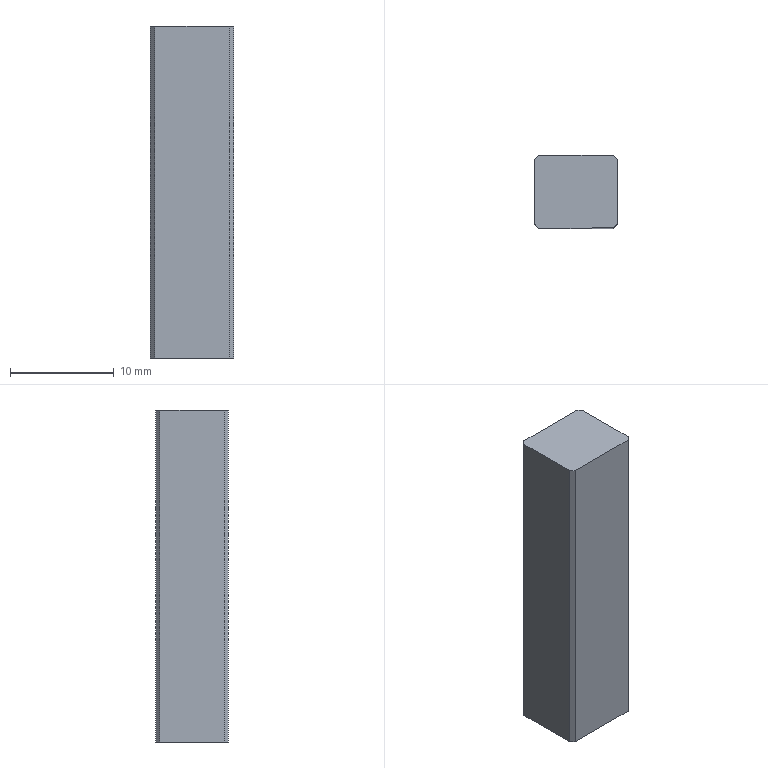Part | STEP file | PLAIN_PARALLEL_KEYS-1-SOLID1 | 1 solid | 10 faces | box 8.009 x 7.011 x 32 mm | volume 1782 mm3 | plane 10
STEP:
#1=CARTESIAN_POINT('',(0.,0.,0.));
#2=DIRECTION('',(0.,0.,1.));
#3=DIRECTION('',(1.,0.,0.));
#4=AXIS2_PLACEMENT_3D('',#1,#2,#3);
#5=CARTESIAN_POINT('',(-3.61,6.995,55.));
#6=VERTEX_POINT('',#5);
#7=CARTESIAN_POINT('',(-3.61,6.995,23.));
#8=VERTEX_POINT('',#7);
#9=CARTESIAN_POINT('',(-3.61,6.995,51.));
#10=DIRECTION('',(0.,0.,-1.));
#11=VECTOR('',#10,1.);
#12=LINE('',#9,#11);
#13=CARTESIAN_POINT('',(-0.01045,7.,51.));
#14=DIRECTION('',(0.001493,-1.,0.));
#15=DIRECTION('',(1.,0.001493,0.));
#16=AXIS2_PLACEMENT_3D('',#13,#14,#15);
#17=PLANE('',#16);
#18=CARTESIAN_POINT('',(-3.6,0.));
#19=DIRECTION('',(0.,-1.));
#20=VECTOR('',#19,1.);
#21=LINE('',#18,#20);
#22=(GEOMETRIC_REPRESENTATION_CONTEXT(2)PARAMETRIC_REPRESENTATION_CONTEXT()REPRESENTATION_CONTEXT('',''));
#23=DEFINITIONAL_REPRESENTATION('',(#21),#22);
#24=PCURVE('',#17,#23);
#25=CARTESIAN_POINT('',(-4.011,7.394,51.));
#26=DIRECTION('',(-0.7061,-0.7082,0.));
#27=DIRECTION('',(0.7082,-0.7061,0.));
#28=AXIS2_PLACEMENT_3D('',#25,#26,#27);
#29=PLANE('',#28);
#30=CARTESIAN_POINT('',(0.5657,0.));
#31=DIRECTION('',(0.,-1.));
#32=VECTOR('',#31,1.);
#33=LINE('',#30,#32);
#34=(GEOMETRIC_REPRESENTATION_CONTEXT(2)PARAMETRIC_REPRESENTATION_CONTEXT()REPRESENTATION_CONTEXT('',''));
#35=DEFINITIONAL_REPRESENTATION('',(#33),#34);
#36=PCURVE('',#29,#35);
#37=SURFACE_CURVE('',#12,(#24,#36),.PCURVE_S1.);
#38=EDGE_CURVE('',#6,#8,#37,.T.);
#39=ORIENTED_EDGE('',*,*,#38,.T.);
#40=CARTESIAN_POINT('',(3.59,7.005,23.));
#41=VERTEX_POINT('',#40);
#42=CARTESIAN_POINT('',(-0.01045,7.,23.));
#43=DIRECTION('',(1.,0.001493,0.));
#44=VECTOR('',#43,1.);
#45=LINE('',#42,#44);
#46=CARTESIAN_POINT('',(0.,-28.));
#47=DIRECTION('',(1.,0.));
#48=VECTOR('',#47,1.);
#49=LINE('',#46,#48);
#50=(GEOMETRIC_REPRESENTATION_CONTEXT(2)PARAMETRIC_REPRESENTATION_CONTEXT()REPRESENTATION_CONTEXT('',''));
#51=DEFINITIONAL_REPRESENTATION('',(#49),#50);
#52=PCURVE('',#17,#51);
#53=CARTESIAN_POINT('',(-4.021,13.994,23.));
#54=DIRECTION('',(0.,0.,1.));
#55=DIRECTION('',(1.,0.,0.));
#56=AXIS2_PLACEMENT_3D('',#53,#54,#55);
#57=PLANE('',#56);
#58=CARTESIAN_POINT('',(4.01,-6.994));
#59=DIRECTION('',(1.,0.001493));
#60=VECTOR('',#59,1.);
#61=LINE('',#58,#60);
#62=(GEOMETRIC_REPRESENTATION_CONTEXT(2)PARAMETRIC_REPRESENTATION_CONTEXT()REPRESENTATION_CONTEXT('',''));
#63=DEFINITIONAL_REPRESENTATION('',(#61),#62);
#64=PCURVE('',#57,#63);
#65=SURFACE_CURVE('',#45,(#52,#64),.PCURVE_S1.);
#66=EDGE_CURVE('',#8,#41,#65,.T.);
#67=ORIENTED_EDGE('',*,*,#66,.T.);
#68=CARTESIAN_POINT('',(3.59,7.005,55.));
#69=VERTEX_POINT('',#68);
#70=CARTESIAN_POINT('',(3.59,7.005,51.));
#71=DIRECTION('',(0.,0.,1.));
#72=VECTOR('',#71,1.);
#73=LINE('',#70,#72);
#74=CARTESIAN_POINT('',(3.6,0.));
#75=DIRECTION('',(0.,1.));
#76=VECTOR('',#75,1.);
#77=LINE('',#74,#76);
#78=(GEOMETRIC_REPRESENTATION_CONTEXT(2)PARAMETRIC_REPRESENTATION_CONTEXT()REPRESENTATION_CONTEXT('',''));
#79=DEFINITIONAL_REPRESENTATION('',(#77),#78);
#80=PCURVE('',#17,#79);
#81=CARTESIAN_POINT('',(3.989,7.406,27.));
#82=DIRECTION('',(0.7082,-0.7061,0.));
#83=DIRECTION('',(0.7061,0.7082,0.));
#84=AXIS2_PLACEMENT_3D('',#81,#82,#83);
#85=PLANE('',#84);
#86=CARTESIAN_POINT('',(-0.5657,24.));
#87=DIRECTION('',(0.,1.));
#88=VECTOR('',#87,1.);
#89=LINE('',#86,#88);
#90=(GEOMETRIC_REPRESENTATION_CONTEXT(2)PARAMETRIC_REPRESENTATION_CONTEXT()REPRESENTATION_CONTEXT('',''));
#91=DEFINITIONAL_REPRESENTATION('',(#89),#90);
#92=PCURVE('',#85,#91);
#93=SURFACE_CURVE('',#73,(#80,#92),.PCURVE_S1.);
#94=EDGE_CURVE('',#41,#69,#93,.T.);
#95=ORIENTED_EDGE('',*,*,#94,.T.);
#96=CARTESIAN_POINT('',(-0.01045,7.,55.));
#97=DIRECTION('',(-1.,-0.001493,0.));
#98=VECTOR('',#97,1.);
#99=LINE('',#96,#98);
#100=CARTESIAN_POINT('',(0.,4.));
#101=DIRECTION('',(-1.,0.));
#102=VECTOR('',#101,1.);
#103=LINE('',#100,#102);
#104=(GEOMETRIC_REPRESENTATION_CONTEXT(2)PARAMETRIC_REPRESENTATION_CONTEXT()REPRESENTATION_CONTEXT('',''));
#105=DEFINITIONAL_REPRESENTATION('',(#103),#104);
#106=PCURVE('',#17,#105);
#107=CARTESIAN_POINT('',(-4.021,13.994,55.));
#108=DIRECTION('',(0.,0.,-1.));
#109=DIRECTION('',(-1.,0.,0.));
#110=AXIS2_PLACEMENT_3D('',#107,#108,#109);
#111=PLANE('',#110);
#112=CARTESIAN_POINT('',(-4.01,-6.994));
#113=DIRECTION('',(1.,-0.001493));
#114=VECTOR('',#113,1.);
#115=LINE('',#112,#114);
#116=(GEOMETRIC_REPRESENTATION_CONTEXT(2)PARAMETRIC_REPRESENTATION_CONTEXT()REPRESENTATION_CONTEXT('',''));
#117=DEFINITIONAL_REPRESENTATION('',(#115),#116);
#118=PCURVE('',#111,#117);
#119=SURFACE_CURVE('',#99,(#106,#118),.PCURVE_S1.);
#120=EDGE_CURVE('',#69,#6,#119,.T.);
#121=ORIENTED_EDGE('',*,*,#120,.T.);
#122=EDGE_LOOP('',(#39,#67,#95,#121));
#123=FACE_BOUND('',#122,.T.);
#124=ADVANCED_FACE('',(#123),#17,.T.);
#125=ORIENTED_EDGE('',*,*,#66,.F.);
#126=CARTESIAN_POINT('',(-4.011,7.394,23.));
#127=VERTEX_POINT('',#126);
#128=CARTESIAN_POINT('',(-4.011,7.394,23.));
#129=DIRECTION('',(0.7082,-0.7061,0.));
#130=VECTOR('',#129,1.);
#131=LINE('',#128,#130);
#132=CARTESIAN_POINT('',(0.009856,-6.6));
#133=DIRECTION('',(0.7082,-0.7061));
#134=VECTOR('',#133,1.);
#135=LINE('',#132,#134);
#136=(GEOMETRIC_REPRESENTATION_CONTEXT(2)PARAMETRIC_REPRESENTATION_CONTEXT()REPRESENTATION_CONTEXT('',''));
#137=DEFINITIONAL_REPRESENTATION('',(#135),#136);
#138=PCURVE('',#57,#137);
#139=CARTESIAN_POINT('',(0.,-28.));
#140=DIRECTION('',(1.,0.));
#141=VECTOR('',#140,1.);
#142=LINE('',#139,#141);
#143=(GEOMETRIC_REPRESENTATION_CONTEXT(2)PARAMETRIC_REPRESENTATION_CONTEXT()REPRESENTATION_CONTEXT('',''));
#144=DEFINITIONAL_REPRESENTATION('',(#142),#143);
#145=PCURVE('',#29,#144);
#146=SURFACE_CURVE('',#131,(#138,#145),.PCURVE_S1.);
#147=EDGE_CURVE('',#127,#8,#146,.T.);
#148=ORIENTED_EDGE('',*,*,#147,.F.);
#149=CARTESIAN_POINT('',(-4.02,13.594,23.));
#150=VERTEX_POINT('',#149);
#151=CARTESIAN_POINT('',(-4.02,13.594,23.));
#152=DIRECTION('',(0.001493,-1.,0.));
#153=VECTOR('',#152,1.);
#154=LINE('',#151,#153);
#155=CARTESIAN_POINT('',(0.0005974,-0.4));
#156=DIRECTION('',(0.001493,-1.));
#157=VECTOR('',#156,1.);
#158=LINE('',#155,#157);
#159=(GEOMETRIC_REPRESENTATION_CONTEXT(2)PARAMETRIC_REPRESENTATION_CONTEXT()REPRESENTATION_CONTEXT('',''));
#160=DEFINITIONAL_REPRESENTATION('',(#158),#159);
#161=PCURVE('',#57,#160);
#162=CARTESIAN_POINT('',(-4.021,13.994,51.));
#163=DIRECTION('',(1.,0.001493,0.));
#164=DIRECTION('',(-0.001493,1.,0.));
#165=AXIS2_PLACEMENT_3D('',#162,#163,#164);
#166=PLANE('',#165);
#167=CARTESIAN_POINT('',(-0.4,-28.));
#168=DIRECTION('',(-1.,0.));
#169=VECTOR('',#168,1.);
#170=LINE('',#167,#169);
#171=(GEOMETRIC_REPRESENTATION_CONTEXT(2)PARAMETRIC_REPRESENTATION_CONTEXT()REPRESENTATION_CONTEXT('',''));
#172=DEFINITIONAL_REPRESENTATION('',(#170),#171);
#173=PCURVE('',#166,#172);
#174=SURFACE_CURVE('',#154,(#161,#173),.PCURVE_S1.);
#175=EDGE_CURVE('',#150,#127,#174,.T.);
#176=ORIENTED_EDGE('',*,*,#175,.F.);
#177=CARTESIAN_POINT('',(-3.621,13.995,23.));
#178=VERTEX_POINT('',#177);
#179=CARTESIAN_POINT('',(-3.621,13.995,23.));
#180=DIRECTION('',(0.7061,0.7082,0.));
#181=VECTOR('',#180,1.);
#182=LINE('',#179,#181);
#183=CARTESIAN_POINT('',(0.4,0.0005974));
#184=DIRECTION('',(0.7061,0.7082));
#185=VECTOR('',#184,1.);
#186=LINE('',#183,#185);
#187=(GEOMETRIC_REPRESENTATION_CONTEXT(2)PARAMETRIC_REPRESENTATION_CONTEXT()REPRESENTATION_CONTEXT('',''));
#188=DEFINITIONAL_REPRESENTATION('',(#186),#187);
#189=PCURVE('',#57,#188);
#190=CARTESIAN_POINT('',(-3.621,13.995,51.));
#191=DIRECTION('',(0.7082,-0.7061,0.));
#192=DIRECTION('',(0.7061,0.7082,0.));
#193=AXIS2_PLACEMENT_3D('',#190,#191,#192);
#194=PLANE('',#193);
#195=CARTESIAN_POINT('',(0.,-28.));
#196=DIRECTION('',(1.,0.));
#197=VECTOR('',#196,1.);
#198=LINE('',#195,#197);
#199=(GEOMETRIC_REPRESENTATION_CONTEXT(2)PARAMETRIC_REPRESENTATION_CONTEXT()REPRESENTATION_CONTEXT('',''));
#200=DEFINITIONAL_REPRESENTATION('',(#198),#199);
#201=PCURVE('',#194,#200);
#202=SURFACE_CURVE('',#182,(#189,#201),.PCURVE_S1.);
#203=EDGE_CURVE('',#150,#178,#202,.T.);
#204=ORIENTED_EDGE('',*,*,#203,.T.);
#205=CARTESIAN_POINT('',(3.579,14.005,23.));
#206=VERTEX_POINT('',#205);
#207=CARTESIAN_POINT('',(3.579,14.005,23.));
#208=DIRECTION('',(-1.,-0.001493,0.));
#209=VECTOR('',#208,1.);
#210=LINE('',#207,#209);
#211=CARTESIAN_POINT('',(7.6,0.01135));
#212=DIRECTION('',(-1.,-0.001493));
#213=VECTOR('',#212,1.);
#214=LINE('',#211,#213);
#215=(GEOMETRIC_REPRESENTATION_CONTEXT(2)PARAMETRIC_REPRESENTATION_CONTEXT()REPRESENTATION_CONTEXT('',''));
#216=DEFINITIONAL_REPRESENTATION('',(#214),#215);
#217=PCURVE('',#57,#216);
#218=CARTESIAN_POINT('',(-0.02091,14.,51.));
#219=DIRECTION('',(0.001493,-1.,0.));
#220=DIRECTION('',(1.,0.001493,0.));
#221=AXIS2_PLACEMENT_3D('',#218,#219,#220);
#222=PLANE('',#221);
#223=CARTESIAN_POINT('',(3.6,-28.));
#224=DIRECTION('',(-1.,0.));
#225=VECTOR('',#224,1.);
#226=LINE('',#223,#225);
#227=(GEOMETRIC_REPRESENTATION_CONTEXT(2)PARAMETRIC_REPRESENTATION_CONTEXT()REPRESENTATION_CONTEXT('',''));
#228=DEFINITIONAL_REPRESENTATION('',(#226),#227);
#229=PCURVE('',#222,#228);
#230=SURFACE_CURVE('',#210,(#217,#229),.PCURVE_S1.);
#231=EDGE_CURVE('',#206,#178,#230,.T.);
#232=ORIENTED_EDGE('',*,*,#231,.F.);
#233=CARTESIAN_POINT('',(3.98,13.606,23.));
#234=VERTEX_POINT('',#233);
#235=CARTESIAN_POINT('',(3.579,14.005,23.));
#236=DIRECTION('',(0.7082,-0.7061,0.));
#237=VECTOR('',#236,1.);
#238=LINE('',#235,#237);
#239=CARTESIAN_POINT('',(7.6,0.01135));
#240=DIRECTION('',(0.7082,-0.7061));
#241=VECTOR('',#240,1.);
#242=LINE('',#239,#241);
#243=(GEOMETRIC_REPRESENTATION_CONTEXT(2)PARAMETRIC_REPRESENTATION_CONTEXT()REPRESENTATION_CONTEXT('',''));
#244=DEFINITIONAL_REPRESENTATION('',(#242),#243);
#245=PCURVE('',#57,#244);
#246=CARTESIAN_POINT('',(3.579,14.005,51.));
#247=DIRECTION('',(-0.7061,-0.7082,0.));
#248=DIRECTION('',(0.7082,-0.7061,0.));
#249=AXIS2_PLACEMENT_3D('',#246,#247,#248);
#250=PLANE('',#249);
#251=CARTESIAN_POINT('',(0.,-28.));
#252=DIRECTION('',(1.,0.));
#253=VECTOR('',#252,1.);
#254=LINE('',#251,#253);
#255=(GEOMETRIC_REPRESENTATION_CONTEXT(2)PARAMETRIC_REPRESENTATION_CONTEXT()REPRESENTATION_CONTEXT('',''));
#256=DEFINITIONAL_REPRESENTATION('',(#254),#255);
#257=PCURVE('',#250,#256);
#258=SURFACE_CURVE('',#238,(#245,#257),.PCURVE_S1.);
#259=EDGE_CURVE('',#206,#234,#258,.T.);
#260=ORIENTED_EDGE('',*,*,#259,.T.);
#261=CARTESIAN_POINT('',(3.989,7.406,23.));
#262=VERTEX_POINT('',#261);
#263=CARTESIAN_POINT('',(3.989,7.406,23.));
#264=DIRECTION('',(-0.001493,1.,0.));
#265=VECTOR('',#264,1.);
#266=LINE('',#263,#265);
#267=CARTESIAN_POINT('',(8.01,-6.588));
#268=DIRECTION('',(-0.001493,1.));
#269=VECTOR('',#268,1.);
#270=LINE('',#267,#269);
#271=(GEOMETRIC_REPRESENTATION_CONTEXT(2)PARAMETRIC_REPRESENTATION_CONTEXT()REPRESENTATION_CONTEXT('',''));
#272=DEFINITIONAL_REPRESENTATION('',(#270),#271);
#273=PCURVE('',#57,#272);
#274=CARTESIAN_POINT('',(3.979,14.006,27.));
#275=DIRECTION('',(-1.,-0.001493,0.));
#276=DIRECTION('',(0.001493,-1.,0.));
#277=AXIS2_PLACEMENT_3D('',#274,#275,#276);
#278=PLANE('',#277);
#279=CARTESIAN_POINT('',(6.6,-4.));
#280=DIRECTION('',(-1.,0.));
#281=VECTOR('',#280,1.);
#282=LINE('',#279,#281);
#283=(GEOMETRIC_REPRESENTATION_CONTEXT(2)PARAMETRIC_REPRESENTATION_CONTEXT()REPRESENTATION_CONTEXT('',''));
#284=DEFINITIONAL_REPRESENTATION('',(#282),#283);
#285=PCURVE('',#278,#284);
#286=SURFACE_CURVE('',#266,(#273,#285),.PCURVE_S1.);
#287=EDGE_CURVE('',#262,#234,#286,.T.);
#288=ORIENTED_EDGE('',*,*,#287,.F.);
#289=CARTESIAN_POINT('',(3.59,7.005,23.));
#290=DIRECTION('',(0.7061,0.7082,0.));
#291=VECTOR('',#290,1.);
#292=LINE('',#289,#291);
#293=CARTESIAN_POINT('',(7.61,-6.989));
#294=DIRECTION('',(0.7061,0.7082));
#295=VECTOR('',#294,1.);
#296=LINE('',#293,#295);
#297=(GEOMETRIC_REPRESENTATION_CONTEXT(2)PARAMETRIC_REPRESENTATION_CONTEXT()REPRESENTATION_CONTEXT('',''));
#298=DEFINITIONAL_REPRESENTATION('',(#296),#297);
#299=PCURVE('',#57,#298);
#300=CARTESIAN_POINT('',(-0.5657,-4.));
#301=DIRECTION('',(1.,0.));
#302=VECTOR('',#301,1.);
#303=LINE('',#300,#302);
#304=(GEOMETRIC_REPRESENTATION_CONTEXT(2)PARAMETRIC_REPRESENTATION_CONTEXT()REPRESENTATION_CONTEXT('',''));
#305=DEFINITIONAL_REPRESENTATION('',(#303),#304);
#306=PCURVE('',#85,#305);
#307=SURFACE_CURVE('',#292,(#299,#306),.PCURVE_S1.);
#308=EDGE_CURVE('',#41,#262,#307,.T.);
#309=ORIENTED_EDGE('',*,*,#308,.F.);
#310=EDGE_LOOP('',(#125,#148,#176,#204,#232,#260,#288,#309));
#311=FACE_BOUND('',#310,.T.);
#312=ADVANCED_FACE('',(#311),#57,.F.);
#313=CARTESIAN_POINT('',(-4.011,7.394,55.));
#314=VERTEX_POINT('',#313);
#315=CARTESIAN_POINT('',(-4.011,7.394,51.));
#316=DIRECTION('',(0.,0.,-1.));
#317=VECTOR('',#316,1.);
#318=LINE('',#315,#317);
#319=CARTESIAN_POINT('',(0.,0.));
#320=DIRECTION('',(0.,-1.));
#321=VECTOR('',#320,1.);
#322=LINE('',#319,#321);
#323=(GEOMETRIC_REPRESENTATION_CONTEXT(2)PARAMETRIC_REPRESENTATION_CONTEXT()REPRESENTATION_CONTEXT('',''));
#324=DEFINITIONAL_REPRESENTATION('',(#322),#323);
#325=PCURVE('',#29,#324);
#326=CARTESIAN_POINT('',(-6.6,0.));
#327=DIRECTION('',(0.,-1.));
#328=VECTOR('',#327,1.);
#329=LINE('',#326,#328);
#330=(GEOMETRIC_REPRESENTATION_CONTEXT(2)PARAMETRIC_REPRESENTATION_CONTEXT()REPRESENTATION_CONTEXT('',''));
#331=DEFINITIONAL_REPRESENTATION('',(#329),#330);
#332=PCURVE('',#166,#331);
#333=SURFACE_CURVE('',#318,(#325,#332),.PCURVE_S1.);
#334=EDGE_CURVE('',#314,#127,#333,.T.);
#335=ORIENTED_EDGE('',*,*,#334,.T.);
#336=ORIENTED_EDGE('',*,*,#147,.T.);
#337=ORIENTED_EDGE('',*,*,#38,.F.);
#338=CARTESIAN_POINT('',(-4.011,7.394,55.));
#339=DIRECTION('',(-0.7082,0.7061,0.));
#340=VECTOR('',#339,1.);
#341=LINE('',#338,#340);
#342=CARTESIAN_POINT('',(0.,4.));
#343=DIRECTION('',(-1.,0.));
#344=VECTOR('',#343,1.);
#345=LINE('',#342,#344);
#346=(GEOMETRIC_REPRESENTATION_CONTEXT(2)PARAMETRIC_REPRESENTATION_CONTEXT()REPRESENTATION_CONTEXT('',''));
#347=DEFINITIONAL_REPRESENTATION('',(#345),#346);
#348=PCURVE('',#29,#347);
#349=CARTESIAN_POINT('',(-0.009856,-6.6));
#350=DIRECTION('',(0.7082,0.7061));
#351=VECTOR('',#350,1.);
#352=LINE('',#349,#351);
#353=(GEOMETRIC_REPRESENTATION_CONTEXT(2)PARAMETRIC_REPRESENTATION_CONTEXT()REPRESENTATION_CONTEXT('',''));
#354=DEFINITIONAL_REPRESENTATION('',(#352),#353);
#355=PCURVE('',#111,#354);
#356=SURFACE_CURVE('',#341,(#348,#355),.PCURVE_S1.);
#357=EDGE_CURVE('',#6,#314,#356,.T.);
#358=ORIENTED_EDGE('',*,*,#357,.T.);
#359=EDGE_LOOP('',(#335,#336,#337,#358));
#360=FACE_BOUND('',#359,.T.);
#361=ADVANCED_FACE('',(#360),#29,.T.);
#362=CARTESIAN_POINT('',(3.98,13.606,55.));
#363=VERTEX_POINT('',#362);
#364=CARTESIAN_POINT('',(3.989,7.406,55.));
#365=VERTEX_POINT('',#364);
#366=CARTESIAN_POINT('',(3.98,13.606,55.));
#367=DIRECTION('',(0.001493,-1.,0.));
#368=VECTOR('',#367,1.);
#369=LINE('',#366,#368);
#370=CARTESIAN_POINT('',(-8.001,-0.3881));
#371=DIRECTION('',(-0.001493,-1.));
#372=VECTOR('',#371,1.);
#373=LINE('',#370,#372);
#374=(GEOMETRIC_REPRESENTATION_CONTEXT(2)PARAMETRIC_REPRESENTATION_CONTEXT()REPRESENTATION_CONTEXT('',''));
#375=DEFINITIONAL_REPRESENTATION('',(#373),#374);
#376=PCURVE('',#111,#375);
#377=CARTESIAN_POINT('',(0.4,28.));
#378=DIRECTION('',(1.,0.));
#379=VECTOR('',#378,1.);
#380=LINE('',#377,#379);
#381=(GEOMETRIC_REPRESENTATION_CONTEXT(2)PARAMETRIC_REPRESENTATION_CONTEXT()REPRESENTATION_CONTEXT('',''));
#382=DEFINITIONAL_REPRESENTATION('',(#380),#381);
#383=PCURVE('',#278,#382);
#384=SURFACE_CURVE('',#369,(#376,#383),.PCURVE_S1.);
#385=EDGE_CURVE('',#363,#365,#384,.T.);
#386=ORIENTED_EDGE('',*,*,#385,.F.);
#387=CARTESIAN_POINT('',(3.579,14.005,55.));
#388=VERTEX_POINT('',#387);
#389=CARTESIAN_POINT('',(3.579,14.005,55.));
#390=DIRECTION('',(-0.7082,0.7061,0.));
#391=VECTOR('',#390,1.);
#392=LINE('',#389,#391);
#393=CARTESIAN_POINT('',(-7.6,0.01135));
#394=DIRECTION('',(0.7082,0.7061));
#395=VECTOR('',#394,1.);
#396=LINE('',#393,#395);
#397=(GEOMETRIC_REPRESENTATION_CONTEXT(2)PARAMETRIC_REPRESENTATION_CONTEXT()REPRESENTATION_CONTEXT('',''));
#398=DEFINITIONAL_REPRESENTATION('',(#396),#397);
#399=PCURVE('',#111,#398);
#400=CARTESIAN_POINT('',(0.,4.));
#401=DIRECTION('',(-1.,0.));
#402=VECTOR('',#401,1.);
#403=LINE('',#400,#402);
#404=(GEOMETRIC_REPRESENTATION_CONTEXT(2)PARAMETRIC_REPRESENTATION_CONTEXT()REPRESENTATION_CONTEXT('',''));
#405=DEFINITIONAL_REPRESENTATION('',(#403),#404);
#406=PCURVE('',#250,#405);
#407=SURFACE_CURVE('',#392,(#399,#406),.PCURVE_S1.);
#408=EDGE_CURVE('',#363,#388,#407,.T.);
#409=ORIENTED_EDGE('',*,*,#408,.T.);
#410=CARTESIAN_POINT('',(-3.621,13.995,55.));
#411=VERTEX_POINT('',#410);
#412=CARTESIAN_POINT('',(-3.621,13.995,55.));
#413=DIRECTION('',(1.,0.001493,0.));
#414=VECTOR('',#413,1.);
#415=LINE('',#412,#414);
#416=CARTESIAN_POINT('',(-0.4,0.0005974));
#417=DIRECTION('',(-1.,0.001493));
#418=VECTOR('',#417,1.);
#419=LINE('',#416,#418);
#420=(GEOMETRIC_REPRESENTATION_CONTEXT(2)PARAMETRIC_REPRESENTATION_CONTEXT()REPRESENTATION_CONTEXT('',''));
#421=DEFINITIONAL_REPRESENTATION('',(#419),#420);
#422=PCURVE('',#111,#421);
#423=CARTESIAN_POINT('',(-3.6,4.));
#424=DIRECTION('',(1.,0.));
#425=VECTOR('',#424,1.);
#426=LINE('',#423,#425);
#427=(GEOMETRIC_REPRESENTATION_CONTEXT(2)PARAMETRIC_REPRESENTATION_CONTEXT()REPRESENTATION_CONTEXT('',''));
#428=DEFINITIONAL_REPRESENTATION('',(#426),#427);
#429=PCURVE('',#222,#428);
#430=SURFACE_CURVE('',#415,(#422,#429),.PCURVE_S1.);
#431=EDGE_CURVE('',#411,#388,#430,.T.);
#432=ORIENTED_EDGE('',*,*,#431,.F.);
#433=CARTESIAN_POINT('',(-4.02,13.594,55.));
#434=VERTEX_POINT('',#433);
#435=CARTESIAN_POINT('',(-3.621,13.995,55.));
#436=DIRECTION('',(-0.7061,-0.7082,0.));
#437=VECTOR('',#436,1.);
#438=LINE('',#435,#437);
#439=CARTESIAN_POINT('',(-0.4,0.0005974));
#440=DIRECTION('',(0.7061,-0.7082));
#441=VECTOR('',#440,1.);
#442=LINE('',#439,#441);
#443=(GEOMETRIC_REPRESENTATION_CONTEXT(2)PARAMETRIC_REPRESENTATION_CONTEXT()REPRESENTATION_CONTEXT('',''));
#444=DEFINITIONAL_REPRESENTATION('',(#442),#443);
#445=PCURVE('',#111,#444);
#446=CARTESIAN_POINT('',(0.,4.));
#447=DIRECTION('',(-1.,0.));
#448=VECTOR('',#447,1.);
#449=LINE('',#446,#448);
#450=(GEOMETRIC_REPRESENTATION_CONTEXT(2)PARAMETRIC_REPRESENTATION_CONTEXT()REPRESENTATION_CONTEXT('',''));
#451=DEFINITIONAL_REPRESENTATION('',(#449),#450);
#452=PCURVE('',#194,#451);
#453=SURFACE_CURVE('',#438,(#445,#452),.PCURVE_S1.);
#454=EDGE_CURVE('',#411,#434,#453,.T.);
#455=ORIENTED_EDGE('',*,*,#454,.T.);
#456=CARTESIAN_POINT('',(-4.011,7.394,55.));
#457=DIRECTION('',(-0.001493,1.,0.));
#458=VECTOR('',#457,1.);
#459=LINE('',#456,#458);
#460=CARTESIAN_POINT('',(-0.009856,-6.6));
#461=DIRECTION('',(0.001493,1.));
#462=VECTOR('',#461,1.);
#463=LINE('',#460,#462);
#464=(GEOMETRIC_REPRESENTATION_CONTEXT(2)PARAMETRIC_REPRESENTATION_CONTEXT()REPRESENTATION_CONTEXT('',''));
#465=DEFINITIONAL_REPRESENTATION('',(#463),#464);
#466=PCURVE('',#111,#465);
#467=CARTESIAN_POINT('',(-6.6,4.));
#468=DIRECTION('',(1.,0.));
#469=VECTOR('',#468,1.);
#470=LINE('',#467,#469);
#471=(GEOMETRIC_REPRESENTATION_CONTEXT(2)PARAMETRIC_REPRESENTATION_CONTEXT()REPRESENTATION_CONTEXT('',''));
#472=DEFINITIONAL_REPRESENTATION('',(#470),#471);
#473=PCURVE('',#166,#472);
#474=SURFACE_CURVE('',#459,(#466,#473),.PCURVE_S1.);
#475=EDGE_CURVE('',#314,#434,#474,.T.);
#476=ORIENTED_EDGE('',*,*,#475,.F.);
#477=ORIENTED_EDGE('',*,*,#357,.F.);
#478=ORIENTED_EDGE('',*,*,#120,.F.);
#479=CARTESIAN_POINT('',(3.989,7.406,55.));
#480=DIRECTION('',(-0.7061,-0.7082,0.));
#481=VECTOR('',#480,1.);
#482=LINE('',#479,#481);
#483=CARTESIAN_POINT('',(-8.01,-6.588));
#484=DIRECTION('',(0.7061,-0.7082));
#485=VECTOR('',#484,1.);
#486=LINE('',#483,#485);
#487=(GEOMETRIC_REPRESENTATION_CONTEXT(2)PARAMETRIC_REPRESENTATION_CONTEXT()REPRESENTATION_CONTEXT('',''));
#488=DEFINITIONAL_REPRESENTATION('',(#486),#487);
#489=PCURVE('',#111,#488);
#490=CARTESIAN_POINT('',(0.,28.));
#491=DIRECTION('',(-1.,0.));
#492=VECTOR('',#491,1.);
#493=LINE('',#490,#492);
#494=(GEOMETRIC_REPRESENTATION_CONTEXT(2)PARAMETRIC_REPRESENTATION_CONTEXT()REPRESENTATION_CONTEXT('',''));
#495=DEFINITIONAL_REPRESENTATION('',(#493),#494);
#496=PCURVE('',#85,#495);
#497=SURFACE_CURVE('',#482,(#489,#496),.PCURVE_S1.);
#498=EDGE_CURVE('',#365,#69,#497,.T.);
#499=ORIENTED_EDGE('',*,*,#498,.F.);
#500=EDGE_LOOP('',(#386,#409,#432,#455,#476,#477,#478,#499));
#501=FACE_BOUND('',#500,.T.);
#502=ADVANCED_FACE('',(#501),#111,.F.);
#503=CARTESIAN_POINT('',(3.989,7.406,27.));
#504=DIRECTION('',(0.,0.,1.));
#505=VECTOR('',#504,1.);
#506=LINE('',#503,#505);
#507=CARTESIAN_POINT('',(0.,0.));
#508=DIRECTION('',(0.,1.));
#509=VECTOR('',#508,1.);
#510=LINE('',#507,#509);
#511=(GEOMETRIC_REPRESENTATION_CONTEXT(2)PARAMETRIC_REPRESENTATION_CONTEXT()REPRESENTATION_CONTEXT('',''));
#512=DEFINITIONAL_REPRESENTATION('',(#510),#511);
#513=PCURVE('',#85,#512);
#514=CARTESIAN_POINT('',(6.6,0.));
#515=DIRECTION('',(0.,1.));
#516=VECTOR('',#515,1.);
#517=LINE('',#514,#516);
#518=(GEOMETRIC_REPRESENTATION_CONTEXT(2)PARAMETRIC_REPRESENTATION_CONTEXT()REPRESENTATION_CONTEXT('',''));
#519=DEFINITIONAL_REPRESENTATION('',(#517),#518);
#520=PCURVE('',#278,#519);
#521=SURFACE_CURVE('',#506,(#513,#520),.PCURVE_S1.);
#522=EDGE_CURVE('',#262,#365,#521,.T.);
#523=ORIENTED_EDGE('',*,*,#522,.T.);
#524=ORIENTED_EDGE('',*,*,#498,.T.);
#525=ORIENTED_EDGE('',*,*,#94,.F.);
#526=ORIENTED_EDGE('',*,*,#308,.T.);
#527=EDGE_LOOP('',(#523,#524,#525,#526));
#528=FACE_BOUND('',#527,.T.);
#529=ADVANCED_FACE('',(#528),#85,.T.);
#530=ORIENTED_EDGE('',*,*,#175,.T.);
#531=ORIENTED_EDGE('',*,*,#334,.F.);
#532=ORIENTED_EDGE('',*,*,#475,.T.);
#533=CARTESIAN_POINT('',(-4.02,13.594,51.));
#534=DIRECTION('',(0.,0.,1.));
#535=VECTOR('',#534,1.);
#536=LINE('',#533,#535);
#537=CARTESIAN_POINT('',(-0.4,0.));
#538=DIRECTION('',(0.,1.));
#539=VECTOR('',#538,1.);
#540=LINE('',#537,#539);
#541=(GEOMETRIC_REPRESENTATION_CONTEXT(2)PARAMETRIC_REPRESENTATION_CONTEXT()REPRESENTATION_CONTEXT('',''));
#542=DEFINITIONAL_REPRESENTATION('',(#540),#541);
#543=PCURVE('',#166,#542);
#544=CARTESIAN_POINT('',(-0.5657,0.));
#545=DIRECTION('',(0.,1.));
#546=VECTOR('',#545,1.);
#547=LINE('',#544,#546);
#548=(GEOMETRIC_REPRESENTATION_CONTEXT(2)PARAMETRIC_REPRESENTATION_CONTEXT()REPRESENTATION_CONTEXT('',''));
#549=DEFINITIONAL_REPRESENTATION('',(#547),#548);
#550=PCURVE('',#194,#549);
#551=SURFACE_CURVE('',#536,(#543,#550),.PCURVE_S1.);
#552=EDGE_CURVE('',#150,#434,#551,.T.);
#553=ORIENTED_EDGE('',*,*,#552,.F.);
#554=EDGE_LOOP('',(#530,#531,#532,#553));
#555=FACE_BOUND('',#554,.T.);
#556=ADVANCED_FACE('',(#555),#166,.F.);
#557=ORIENTED_EDGE('',*,*,#231,.T.);
#558=CARTESIAN_POINT('',(-3.621,13.995,51.));
#559=DIRECTION('',(0.,0.,-1.));
#560=VECTOR('',#559,1.);
#561=LINE('',#558,#560);
#562=CARTESIAN_POINT('',(-3.6,0.));
#563=DIRECTION('',(0.,-1.));
#564=VECTOR('',#563,1.);
#565=LINE('',#562,#564);
#566=(GEOMETRIC_REPRESENTATION_CONTEXT(2)PARAMETRIC_REPRESENTATION_CONTEXT()REPRESENTATION_CONTEXT('',''));
#567=DEFINITIONAL_REPRESENTATION('',(#565),#566);
#568=PCURVE('',#222,#567);
#569=CARTESIAN_POINT('',(0.,0.));
#570=DIRECTION('',(0.,-1.));
#571=VECTOR('',#570,1.);
#572=LINE('',#569,#571);
#573=(GEOMETRIC_REPRESENTATION_CONTEXT(2)PARAMETRIC_REPRESENTATION_CONTEXT()REPRESENTATION_CONTEXT('',''));
#574=DEFINITIONAL_REPRESENTATION('',(#572),#573);
#575=PCURVE('',#194,#574);
#576=SURFACE_CURVE('',#561,(#568,#575),.PCURVE_S1.);
#577=EDGE_CURVE('',#411,#178,#576,.T.);
#578=ORIENTED_EDGE('',*,*,#577,.F.);
#579=ORIENTED_EDGE('',*,*,#431,.T.);
#580=CARTESIAN_POINT('',(3.579,14.005,51.));
#581=DIRECTION('',(0.,0.,1.));
#582=VECTOR('',#581,1.);
#583=LINE('',#580,#582);
#584=CARTESIAN_POINT('',(3.6,0.));
#585=DIRECTION('',(0.,1.));
#586=VECTOR('',#585,1.);
#587=LINE('',#584,#586);
#588=(GEOMETRIC_REPRESENTATION_CONTEXT(2)PARAMETRIC_REPRESENTATION_CONTEXT()REPRESENTATION_CONTEXT('',''));
#589=DEFINITIONAL_REPRESENTATION('',(#587),#588);
#590=PCURVE('',#222,#589);
#591=CARTESIAN_POINT('',(0.,0.));
#592=DIRECTION('',(0.,1.));
#593=VECTOR('',#592,1.);
#594=LINE('',#591,#593);
#595=(GEOMETRIC_REPRESENTATION_CONTEXT(2)PARAMETRIC_REPRESENTATION_CONTEXT()REPRESENTATION_CONTEXT('',''));
#596=DEFINITIONAL_REPRESENTATION('',(#594),#595);
#597=PCURVE('',#250,#596);
#598=SURFACE_CURVE('',#583,(#590,#597),.PCURVE_S1.);
#599=EDGE_CURVE('',#206,#388,#598,.T.);
#600=ORIENTED_EDGE('',*,*,#599,.F.);
#601=EDGE_LOOP('',(#557,#578,#579,#600));
#602=FACE_BOUND('',#601,.T.);
#603=ADVANCED_FACE('',(#602),#222,.F.);
#604=ORIENTED_EDGE('',*,*,#287,.T.);
#605=CARTESIAN_POINT('',(3.98,13.606,27.));
#606=DIRECTION('',(0.,0.,-1.));
#607=VECTOR('',#606,1.);
#608=LINE('',#605,#607);
#609=CARTESIAN_POINT('',(0.4,0.));
#610=DIRECTION('',(0.,-1.));
#611=VECTOR('',#610,1.);
#612=LINE('',#609,#611);
#613=(GEOMETRIC_REPRESENTATION_CONTEXT(2)PARAMETRIC_REPRESENTATION_CONTEXT()REPRESENTATION_CONTEXT('',''));
#614=DEFINITIONAL_REPRESENTATION('',(#612),#613);
#615=PCURVE('',#278,#614);
#616=CARTESIAN_POINT('',(0.5657,-24.));
#617=DIRECTION('',(0.,-1.));
#618=VECTOR('',#617,1.);
#619=LINE('',#616,#618);
#620=(GEOMETRIC_REPRESENTATION_CONTEXT(2)PARAMETRIC_REPRESENTATION_CONTEXT()REPRESENTATION_CONTEXT('',''));
#621=DEFINITIONAL_REPRESENTATION('',(#619),#620);
#622=PCURVE('',#250,#621);
#623=SURFACE_CURVE('',#608,(#615,#622),.PCURVE_S1.);
#624=EDGE_CURVE('',#363,#234,#623,.T.);
#625=ORIENTED_EDGE('',*,*,#624,.F.);
#626=ORIENTED_EDGE('',*,*,#385,.T.);
#627=ORIENTED_EDGE('',*,*,#522,.F.);
#628=EDGE_LOOP('',(#604,#625,#626,#627));
#629=FACE_BOUND('',#628,.T.);
#630=ADVANCED_FACE('',(#629),#278,.F.);
#631=ORIENTED_EDGE('',*,*,#454,.F.);
#632=ORIENTED_EDGE('',*,*,#577,.T.);
#633=ORIENTED_EDGE('',*,*,#203,.F.);
#634=ORIENTED_EDGE('',*,*,#552,.T.);
#635=EDGE_LOOP('',(#631,#632,#633,#634));
#636=FACE_BOUND('',#635,.T.);
#637=ADVANCED_FACE('',(#636),#194,.F.);
#638=ORIENTED_EDGE('',*,*,#259,.F.);
#639=ORIENTED_EDGE('',*,*,#599,.T.);
#640=ORIENTED_EDGE('',*,*,#408,.F.);
#641=ORIENTED_EDGE('',*,*,#624,.T.);
#642=EDGE_LOOP('',(#638,#639,#640,#641));
#643=FACE_BOUND('',#642,.T.);
#644=ADVANCED_FACE('',(#643),#250,.F.);
#645=CLOSED_SHELL('',(#124,#312,#361,#502,#529,#556,#603,#630,#637,#644));
#646=MANIFOLD_SOLID_BREP('',#645);
#647=(LENGTH_UNIT()NAMED_UNIT(*)SI_UNIT(.MILLI.,.METRE.));
#648=UNCERTAINTY_MEASURE_WITH_UNIT(LENGTH_MEASURE(0.0000001),#647,'','');
#649=(NAMED_UNIT(*)PLANE_ANGLE_UNIT()SI_UNIT($,.RADIAN.));
#650=(NAMED_UNIT(*)SI_UNIT($,.STERADIAN.)SOLID_ANGLE_UNIT());
#651=(GEOMETRIC_REPRESENTATION_CONTEXT(3)GLOBAL_UNCERTAINTY_ASSIGNED_CONTEXT((#648))GLOBAL_UNIT_ASSIGNED_CONTEXT((#647,#649,#650))REPRESENTATION_CONTEXT('',''));
#652=ADVANCED_BREP_SHAPE_REPRESENTATION('',(#4,#646),#651);